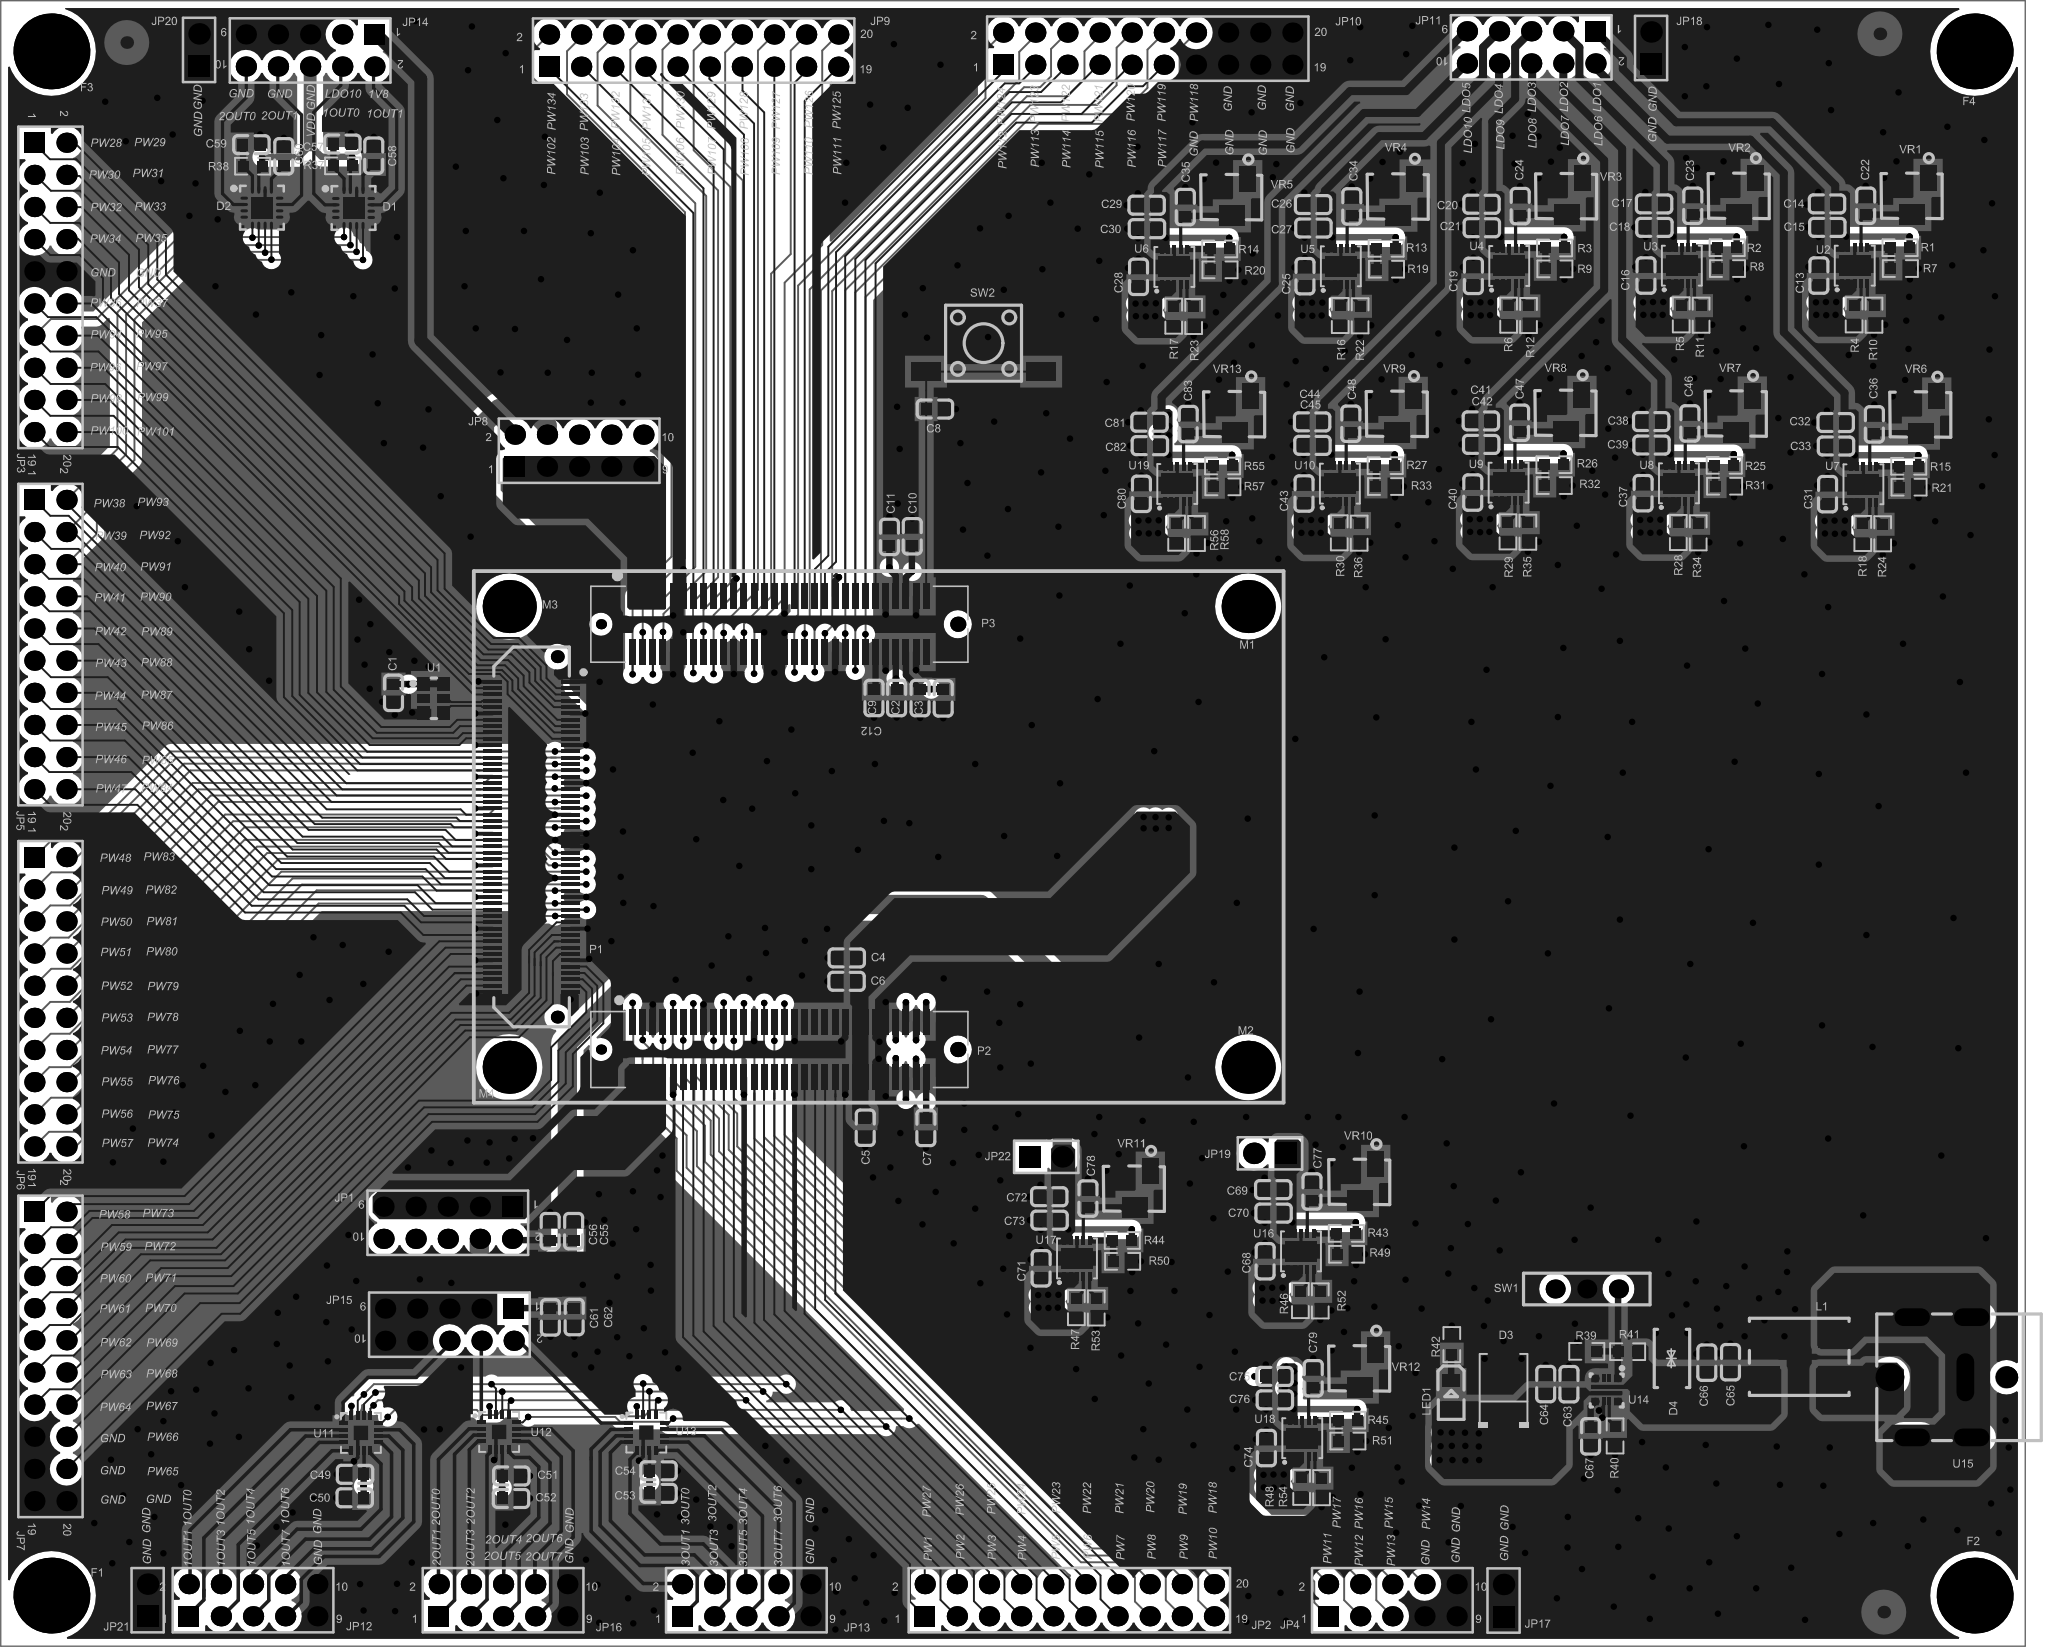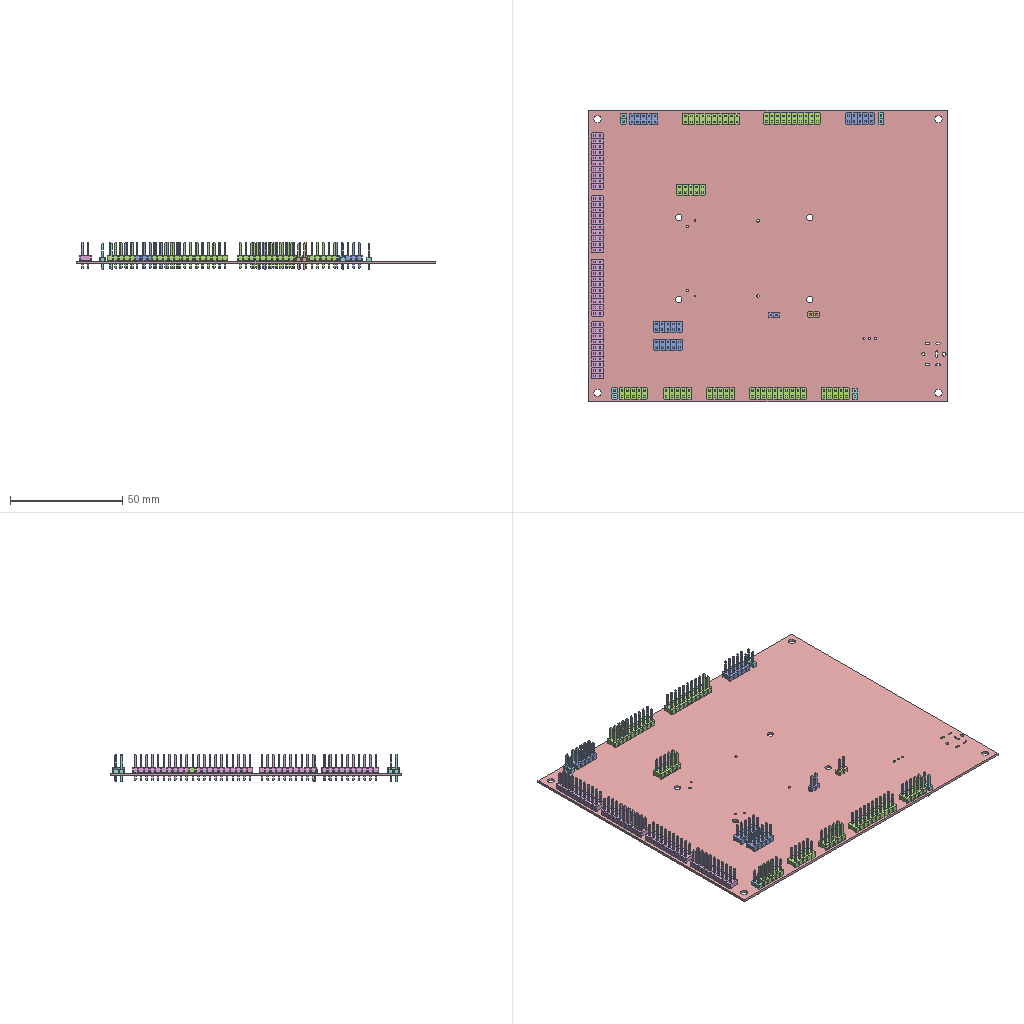Circuit board layout | Altium Designer | box 160 x 130 x 12.2 mm
Layer stack:
# Altium Designer layer stack of  (unit mm; dielectric type: 0 none, 1 core, 2 prepreg, 3 surface material)
index,name,kind,layer,copper_thickness_mm,dielectric_type,dielectric_thickness_mm,dielectric_material,dielectric_constant
0,Top Paste,other,,,,,,
1,Top Overlay,other,,,,,,
2,Top Solder,dielectric,,,3,0.0102,Solder Resist,3.5
3,Top Layer,copper,Top Layer,0.0356,,,,
4,Dielectric1,dielectric,,,1,0.32,FR-4,4.8
5,GND,copper,GND,0.0356,,,,
6,Dielectric2,dielectric,,,2,0.32,FR-4,4.8
7,POWER,copper,POWER,0.0356,,,,
8,Dielectric3,dielectric,,,1,0.32,FR-4,4.8
9,Bottom Layer,copper,Bottom Layer,0.0356,,,,
10,Bottom Solder,dielectric,,,3,0.0102,Solder Resist,3.5
11,Bottom Overlay,other,,,,,,
12,Bottom Paste,other,,,,,,
# drill layer pairs: low layer,high layer
drill_pair,Top Layer,Bottom Layer
Part placement:
Designator,Comment,Layer,Footprint,Center-X(mm),Center-Y(mm),Rotation
C1,X7R  100nF/16V,TopLayer,C0603,31.039,75.311,270
C2,100nF/50V,TopLayer,C0603,72.66,74.915,90
C3,22uF/10V,TopLayer,C0603,74.489,74.889,90
C4,100nF/50V,TopLayer,C0603,66.868,54.372,360
C5,22uF/10V,TopLayer,C0603,68.326,40.97,90
C6,100nF/50V,TopLayer,C0603,66.853,52.527,360
C7,100nF/50V,TopLayer,C0603,73.117,40.955,90
C8,100nF,TopLayer,C0603,73.838,97.739,360
C9,100nF/50V,TopLayer,C0603,70.806,74.915,90
C10,100nF/50V,TopLayer,C0603,72.034,87.681,270
C11,22uF/10V,TopLayer,C0603,70.231,87.63,270
C12,100nF/50V,TopLayer,C0603,69.012,74.905,270
C13,10uF,TopLayer,C0603,143.688,108.28,270
C14,10uF,TopLayer,C0603,144.34,113.944,360
C15,10uF,TopLayer,C0603,144.366,112.09,360
C16,10uF,TopLayer,C0603,130.023,108.28,270
C17,10uF,TopLayer,C0603,130.675,113.944,360
C18,10uF,TopLayer,C0603,130.701,112.09,360
C19,10uF,TopLayer,C0603,116.383,108.255,270
C20,10uF,TopLayer,C0603,117.035,113.919,360
C21,10uF,TopLayer,C0603,117.061,112.065,360
C22,4.7uF,TopLayer,C0603,147.388,113.792,270
C23,4.7uF,TopLayer,C0603,133.723,113.792,270
C24,4.7uF,TopLayer,C0603,120.083,113.767,270
C25,10uF,TopLayer,C0603,103.073,108.229,270
C26,10uF,TopLayer,C0603,103.726,113.894,360
C27,10uF,TopLayer,C0603,103.751,112.039,360
C28,10uF,TopLayer,C0603,89.916,108.179,270
C29,10uF,TopLayer,C0603,90.569,113.843,360
C30,10uF,TopLayer,C0603,90.594,111.989,360
C31,10uF,TopLayer,C0603,144.374,91.008,270
C32,10uF,TopLayer,C0603,145.026,96.672,360
C33,10uF,TopLayer,C0603,145.052,94.818,360
C34,4.7uF,TopLayer,C0603,106.774,113.741,270
C35,4.7uF,TopLayer,C0603,93.617,113.69,270
C36,4.7uF,TopLayer,C0603,148.074,96.52,270
C37,10uF,TopLayer,C0603,129.794,91.084,270
C38,10uF,TopLayer,C0603,130.447,96.749,360
C39,10uF,TopLayer,C0603,130.472,94.894,360
C40,10uF,TopLayer,C0603,116.332,91.135,270
C41,10uF,TopLayer,C0603,116.985,96.799,360
C42,10uF,TopLayer,C0603,117.01,94.945,360
C43,10uF,TopLayer,C0603,102.997,91.059,270
C44,10uF,TopLayer,C0603,103.65,96.723,360
C45,10uF,TopLayer,C0603,103.675,94.869,360
C46,4.7uF,TopLayer,C0603,133.495,96.596,270
C47,4.7uF,TopLayer,C0603,120.033,96.647,270
C48,4.7uF,TopLayer,C0603,106.698,96.571,270
C49,10uF,TopLayer,C0603,28.007,13.574,360
C50,100nF,TopLayer,C0603,27.982,11.72,360
C51,10uF,TopLayer,C0603,40.344,13.452,180
C52,100nF,TopLayer,C0603,40.319,11.674,180
C53,10uF,TopLayer,C0603,51.978,12.08,180
C54,100nF,TopLayer,C0603,51.978,13.858,180
C55,0.1uF/16V,TopLayer,C0603,45.272,32.781,270
C56,0.1uF/16V,TopLayer,C0603,43.418,32.781,270
C57,100nF,TopLayer,C0603,26.991,118.679,180
C58,1.5uF,TopLayer,C0603,29.48,117.765,90
C59,100nF,TopLayer,C0603,19.803,118.628,180
C60,1.5uF,TopLayer,C0603,22.368,117.714,90
C61,10uF,TopLayer,C0603,43.443,25.985,90
C62,10nF,TopLayer,C0603,45.323,26.011,90
C63,22uF/10V,TopLayer,C0603,123.936,20.691,270
C64,22uF/10V,TopLayer,C0603,122.098,20.701,270
C65,X7R 100nF/25V,TopLayer,C0603,136.703,22.428,270
C66,X7R 100nF/25V,TopLayer,C0603,134.832,22.393,270
C67,X7R,TopLayer,C0603,125.654,16.586,90
C68,10uF,TopLayer,C0603,99.924,30.404,270
C69,10uF,TopLayer,C0603,100.576,36.068,360
C70,10uF,TopLayer,C0603,100.602,34.214,360
C71,10uF,TopLayer,C0603,82.22,29.845,270
C72,10uF,TopLayer,C0603,82.872,35.509,360
C73,10uF,TopLayer,C0603,82.898,33.655,360
C74,10uF,TopLayer,C0603,100.025,15.646,270
C75,10uF,TopLayer,C0603,100.678,21.311,360
C76,10uF,TopLayer,C0603,100.703,19.456,360
C77,4.7uF,TopLayer,C0603,103.624,35.916,270
C78,4.7uF,TopLayer,C0603,85.92,35.357,270
C79,4.7uF,TopLayer,C0603,103.726,21.158,270
C80,10uF,TopLayer,C0603,90.145,91.034,270
C81,10uF,TopLayer,C0603,90.797,96.698,360
C82,10uF,TopLayer,C0603,90.823,94.844,360
C83,4.7uF,TopLayer,C0603,93.845,96.545,270
D1,DAC53202,TopLayer,WQFN-16(3x3),27.88,113.624,360
D2,DAC53202,TopLayer,WQFN-16(3x3),20.641,113.65,360
D3,#NAME?,TopLayer,SMB_L4.6-W3.6-LS5.3-RD,118.77,20.345,90
D4,#NAME?,TopLayer,SMA_L4.2-W2.7-LS5.0-BI,132.08,22.733,270
F1,M3,TopLayer,M3,4.004,3.998,0
F2,M3,TopLayer,M3,156.004,3.998,0
F3,M3,TopLayer,M3,4.004,125.998,0
F4,M3,TopLayer,M3,156.004,125.998,0
JP1,Header 5X2,TopLayer,HDR2.54-LI-2x5P,35.331,33.452,180
JP2,Header 2X10,TopLayer,HDR2.54-LI-2x10P,84.455,3.632,360
JP3,Header 2X10,TopLayer,HDR2.54-LI-2x10P,3.928,107.351,270
JP4,Header 5X2,TopLayer,HDR2.54-LI-2x5P,109.982,3.632,360
JP5,Header 2X10,TopLayer,HDR2.54-LI-2x10P,3.928,79.131,270
JP6,Header 2X10,TopLayer,HDR2.54-LI-2x10P,3.928,50.912,270
JP7,Header 2X10,TopLayer,HDR2.54-LI-2x10P,3.928,22.896,270
JP8,Header 5X2,TopLayer,HDR2.54-LI-2x5P,45.711,94.447,360
JP9,Header 2X10,TopLayer,HDR2.54-LI-2x10P,54.762,126.06,360
JP10,Header 2X10,TopLayer,HDR2.54-LI-2x10P,90.653,126.213,360
JP11,Header 5X2,TopLayer,HDR2.54-LI-2x5P,120.955,126.314,180
JP12,Header 5X2,TopLayer,HDR2.54-LI-2x5P,19.939,3.632,360
JP13,Header 5X2,TopLayer,HDR2.54-LI-2x5P,58.928,3.632,360
JP14,Header 5X2,TopLayer,HDR2.54-LI-2x5P,24.451,126.07,180
JP15,Header 5X2,TopLayer,HDR2.54-LI-2x5P,35.458,25.4,180
JP16,Header 5X2,TopLayer,HDR2.54-LI-2x5P,39.7,3.632,360
JP17,HDR-1X2,TopLayer,HDR2.54-LI-2P,118.77,3.607,90
JP18,HDR-1X2,TopLayer,HDR2.54-LI-2P,130.429,126.263,90
JP19,HDR-1X2,TopLayer,HDR2.54-LI-2P,100.305,38.938,180
JP20,HDR-1X2,TopLayer,HDR2.54-LI-2P,15.672,126.111,90
JP21,HDR-1X2,TopLayer,HDR2.54-LI-2P,11.608,3.632,90
JP22,HDR-1X2,TopLayer,HDR2.54-LI-2P,82.626,38.659,360
L1,#NAME?,TopLayer,FILTER-SMD_4P-L7.0-W6.0-TL_SMCM7060,142.138,22.86,180
LED1,#NAME?,TopLayer,LED0805-R-RD,114.63,19.914,270
M1,M2-4-L5-1.6,TopLayer,M2.9,98.587,82.138,0
M2,M2-4-L5-1.6,TopLayer,M2.9,98.587,45.738,0
M3,M2-4-L5-1.6,TopLayer,M2.9,40.187,82.138,0
M4,M2-4-L5-1.6,TopLayer,M2.9,40.187,45.738,0
P1,XMS6302-B,TopLayer,XMS6302-B,41.952,63.938,270
P2,XMS6302-A,TopLayer,XMS6302-A,61.537,47.139,360
P3,XMS6302-C,TopLayer,XMS6302-C,61.537,80.739,360
R1,453k,TopLayer,R0603,150.106,110.49,360
R2,453k,TopLayer,R0603,136.441,110.49,360
R3,453k,TopLayer,R0603,122.801,110.465,360
R4,200k,TopLayer,R0603,146.474,105.181,270
R5,200k,TopLayer,R0603,132.809,105.181,270
R6,200k,TopLayer,R0603,119.169,105.156,270
R7,50k,TopLayer,R0603,150.132,108.839,180
R8,50k,TopLayer,R0603,136.466,108.839,180
R9,50k,TopLayer,R0603,122.827,108.814,180
R10,249R,TopLayer,R0603,148.049,105.156,90
R11,249R,TopLayer,R0603,134.384,105.156,90
R12,249R,TopLayer,R0603,120.744,105.131,90
R13,453k,TopLayer,R0603,109.492,110.439,360
R14,453k,TopLayer,R0603,96.334,110.388,360
R15,453k,TopLayer,R0603,150.792,93.218,360
R16,200k,TopLayer,R0603,105.859,105.131,270
R17,200k,TopLayer,R0603,92.702,105.08,270
R18,200k,TopLayer,R0603,147.16,87.909,270
R19,50k,TopLayer,R0603,109.517,108.788,180
R20,50k,TopLayer,R0603,96.36,108.737,180
R21,50k,TopLayer,R0603,150.817,91.567,180
R22,249R,TopLayer,R0603,107.434,105.105,90
R23,249R,TopLayer,R0603,94.277,105.054,90
R24,249R,TopLayer,R0603,148.735,87.884,90
R25,453k,TopLayer,R0603,136.212,93.294,360
R26,453k,TopLayer,R0603,122.75,93.345,360
R27,453k,TopLayer,R0603,109.415,93.269,360
R28,200k,TopLayer,R0603,132.58,87.986,270
R29,200k,TopLayer,R0603,119.118,88.036,270
R30,200k,TopLayer,R0603,105.783,87.96,270
R31,50k,TopLayer,R0603,136.238,91.643,180
R32,50k,TopLayer,R0603,122.776,91.694,180
R33,50k,TopLayer,R0603,109.441,91.618,180
R34,249R,TopLayer,R0603,134.155,87.96,90
R35,249R,TopLayer,R0603,120.693,88.011,90
R36,249R,TopLayer,R0603,107.358,87.935,90
R37,10K,TopLayer,R0603,27.016,116.952,360
R38,10K,TopLayer,R0603,19.904,116.926,360
R39,357K,TopLayer,R0603,125.349,23.292,180
R40,681O,TopLayer,R0603,127.584,16.612,270
R41,1M,TopLayer,R0603,128.575,23.266,180
R42,10K,TopLayer,R0603,114.681,23.825,270
R43,453k,TopLayer,R0603,106.342,32.614,360
R44,453k,TopLayer,R0603,88.638,32.055,360
R45,453k,TopLayer,R0603,106.444,17.856,360
R46,200k,TopLayer,R0603,102.71,27.305,270
R47,200k,TopLayer,R0603,85.006,26.746,270
R48,200k,TopLayer,R0603,102.811,12.548,270
R49,50k,TopLayer,R0603,106.367,30.963,180
R50,50k,TopLayer,R0603,88.664,30.404,180
R51,50k,TopLayer,R0603,106.469,16.205,180
R52,249R,TopLayer,R0603,104.285,27.28,90
R53,249R,TopLayer,R0603,86.581,26.721,90
R54,249R,TopLayer,R0603,104.386,12.522,90
R55,453k,TopLayer,R0603,96.563,93.243,360
R56,200k,TopLayer,R0603,92.931,87.935,270
R57,50k,TopLayer,R0603,96.588,91.592,180
R58,249R,TopLayer,R0603,94.506,87.909,90
SW1,#NAME?,TopLayer,SW-TH_K3-1204D,125.349,28.219,360
SW2,Key_SMD_6x6x6.5,TopLayer,SW-SMD_4P-L6.0-W6.0-P4.50-LS9.0-2,77.673,102.946,360
U1,SiT9121AI-2B1-XXE100,TopLayer,3225-6p,34.23,74.889,270
U2,#NAME?,TopLayer,DFN-10_L3.0-W3.0-P0.50-BL-EP-3,146.525,109.068,360
U3,#NAME?,TopLayer,DFN-10_L3.0-W3.0-P0.50-BL-EP-3,132.86,109.068,360
U4,#NAME?,TopLayer,DFN-10_L3.0-W3.0-P0.50-BL-EP-3,119.22,109.042,360
U5,#NAME?,TopLayer,DFN-10_L3.0-W3.0-P0.50-BL-EP-3,105.91,109.017,360
U6,#NAME?,TopLayer,DFN-10_L3.0-W3.0-P0.50-BL-EP-3,92.753,108.966,360
U7,#NAME?,TopLayer,DFN-10_L3.0-W3.0-P0.50-BL-EP-3,147.211,91.796,360
U8,#NAME?,TopLayer,DFN-10_L3.0-W3.0-P0.50-BL-EP-3,132.631,91.872,360
U9,#NAME?,TopLayer,DFN-10_L3.0-W3.0-P0.50-BL-EP-3,119.169,91.923,360
U10,#NAME?,TopLayer,DFN-10_L3.0-W3.0-P0.50-BL-EP-3,105.834,91.846,360
U11,DAC60508ZRTER,TopLayer,WQFN-16_L3.0-W3.0-P0.50-BL-EP0.8,28.464,16.85,270
U12,DAC60508ZRTER,TopLayer,WQFN-16_L3.0-W3.0-P0.50-BL-EP0.8,39.386,16.927,270
U13,DAC60508ZRTER,TopLayer,WQFN-16_L3.0-W3.0-P0.50-BL-EP0.8,51.019,16.876,270
U14,#NAME?,TopLayer,VQFN-10_L2.0-W2.0-P0.45-TL,126.898,20.244,270
U15,#NAME?,TopLayer,DC-IN-TH_HX-DC007B-2.5,153.893,21.245,180
U16,#NAME?,TopLayer,DFN-10_L3.0-W3.0-P0.50-BL-EP-3,102.761,31.191,360
U17,#NAME?,TopLayer,DFN-10_L3.0-W3.0-P0.50-BL-EP-3,85.057,30.632,360
U18,#NAME?,TopLayer,DFN-10_L3.0-W3.0-P0.50-BL-EP-3,102.862,16.434,360
U19,#NAME?,TopLayer,DFN-10_L3.0-W3.0-P0.50-BL-EP-3,92.982,91.821,360
VR1,50kO,TopLayer,RES-ADJ-SMD_3224W,151.071,114.554,180
VR2,50kO,TopLayer,RES-ADJ-SMD_3224W,137.406,114.554,180
VR3,50kO,TopLayer,RES-ADJ-SMD_3224W,123.766,114.529,180
VR4,50kO,TopLayer,RES-ADJ-SMD_3224W,110.457,114.503,180
VR5,50kO,TopLayer,RES-ADJ-SMD_3224W,97.3,114.452,180
VR6,50kO,TopLayer,RES-ADJ-SMD_3224W,151.757,97.282,180
VR7,50kO,TopLayer,RES-ADJ-SMD_3224W,137.178,97.358,180
VR8,50kO,TopLayer,RES-ADJ-SMD_3224W,123.716,97.409,180
VR9,50kO,TopLayer,RES-ADJ-SMD_3224W,110.381,97.333,180
VR10,50kO,TopLayer,RES-ADJ-SMD_3224W,107.417,36.652,180
VR11,50kO,TopLayer,RES-ADJ-SMD_3224W,89.603,36.119,180
VR12,50kO,TopLayer,RES-ADJ-SMD_3224W,107.409,21.92,180
VR13,50kO,TopLayer,RES-ADJ-SMD_3224W,97.528,97.307,180
Pad and via stacks:
# Altium Designer via and pad stacks of  (unit mm). Each distinct definition once, with the count of objects using it.
# via: kind,start_layer,end_layer,hole_mm,diameter_mm,mode(0 simple;1 top-mid-bottom;2 full stack),diameter_per_layer,count,example_net
# pad: kind,layer,hole_mm,hole_type(0 round;1 square;2 slot),plating,top_size,top_shape(1 round;2 rect;3 octagon;9 rounded rect),mid_size,bottom_size,mode,footprint,size_per_layer,count,example
pad,Top Layer,0,0,plated,1x1,1,1x1,1x1,0,,,3,MARK
pad,Top Layer,0,0,plated,0.6x0.24,1,0.6x0.24,0.6x0.24,0,WQFN-16(3x3),,16,D2.1
pad,Top Layer,0,0,plated,0.24x0.6,1,0.24x0.6,0.24x0.6,0,WQFN-16(3x3),,16,D2.5
pad,Top Layer,0,0,plated,1.68x1.68,2,1.68x1.68,1.68x1.68,0,WQFN-16(3x3),,2,D2.17
pad,Top Layer,0,0,plated,0.8x0.9,2,0.8x0.9,0.8x0.9,0,C0603,,166,C61.2
pad,Top Layer,0,0,plated,0.8065x0.864,2,0.8065x0.864,0.8065x0.864,0,R0603,,116,R38.2
pad,Top Layer,0,0,plated,0.8x0.8,2,0.8x0.8,0.8x0.8,0,WQFN-16_L3.0-W3.0-P0.50-BL-EP0.8,,3,U13.17
pad,Top Layer,0,0,plated,0.665x0.28,2,0.665x0.28,0.665x0.28,0,WQFN-16_L3.0-W3.0-P0.50-BL-EP0.8,,24,U13.16
pad,Top Layer,0,0,plated,0.28x0.665,2,0.28x0.665,0.28x0.665,0,WQFN-16_L3.0-W3.0-P0.50-BL-EP0.8,,24,U13.12
pad,Top Layer,0,0,plated,1.6x2,2,1.6x2,1.6x2,0,RES-ADJ-SMD_3224W,,13,VR1.2
pad,Top Layer,0,0,plated,2x1.3,2,2x1.3,2x1.3,0,RES-ADJ-SMD_3224W,,26,VR1.3
pad,Top Layer,0,0,plated,2.5x1.6,2,2.5x1.6,2.5x1.6,0,DFN-10_L3.0-W3.0-P0.50-BL-EP-3,,13,U2.11
pad,Top Layer,0,0,plated,0.25x0.65,2,0.25x0.65,0.25x0.65,0,DFN-10_L3.0-W3.0-P0.50-BL-EP-3,,130,U2.10
pad,Top Layer,0,0,plated,2.3x1.5,2,2.3x1.5,2.3x1.5,0,SW-SMD_4P-L6.0-W6.0-P4.50-LS9.0-2,,4,SW2.1
pad,Top Layer,0,0,unplated,0.5x2,2,0.5x2,0.5x2,0,XMS6302-C,,60,P3.C1
pad,Top Layer,0,0,unplated,0.5x2,2,0.5x2,0.5x2,0,XMS6302-A,,60,P2.A3
pad,Top Layer,0,0,plated,0.65x1,2,0.65x1,0.65x1,0,3225-6p,,2,U1.2
pad,Top Layer,0,0,plated,1.05x1,2,1.05x1,1.05x1,0,3225-6p,,4,U1.1
pad,Top Layer,0,0,plated,0.3051x1.448,2,0.3051x1.448,0.3051x1.448,0,XMS6302-B,,100,P1.B36
pad,Top Layer,0,0,plated,2x1.8,2,2x1.8,2x1.8,0,SMA_L4.2-W2.7-LS5.0-BI,,2,D4.2
pad,Top Layer,0,0,plated,2.5x1.75,2,2.5x1.75,2.5x1.75,0,FILTER-SMD_4P-L7.0-W6.0-TL_SMCM7060,,4,L1.1
pad,Top Layer,0,0,plated,2.047x2.192,2,2.047x2.192,2.047x2.192,0,SMB_L4.6-W3.6-LS5.3-RD,,2,D3.1
pad,Top Layer,0,0,plated,1x1.399,2,1x1.399,1x1.399,0,LED0805-R-RD,,2,LED1.1
pad,Top Layer,0,0,plated,0.6x0.6,1,0.6x0.6,0.6x0.6,0,VQFN-10_L2.0-W2.0-P0.45-TL,,4,U14.1
pad,Top Layer,0,0,plated,0.3x2.4,2,0.3x2.4,0.3x2.4,0,VQFN-10_L2.0-W2.0-P0.45-TL,,2,U14.5
pad,Top Layer,0,0,plated,0.25x0.6,2,0.25x0.6,0.25x0.6,0,VQFN-10_L2.0-W2.0-P0.45-TL,,4,U14.2
pad,Multi-Layer,0.9,0,plated,1.6x1.6,1,1.6x1.6,1.6x1.6,0,HDR2.54-LI-2x5P,,81,JP15.10
pad,Multi-Layer,0.9,0,plated,1.6x1.6,2,1.6x1.6,1.6x1.6,0,HDR2.54-LI-2x5P,,9,JP15.1
pad,Multi-Layer,3.2,0,plated,6x6,1,6x6,6x6,0,M3,,4,F1.1
pad,Multi-Layer,0.9,0,plated,1.6x1.6,1,1.6x1.6,1.6x1.6,0,HDR2.54-LI-2x10P,,133,JP10.20
pad,Multi-Layer,0.9,0,plated,1.6x1.6,2,1.6x1.6,1.6x1.6,0,HDR2.54-LI-2x10P,,7,JP10.1
pad,Multi-Layer,1.2,0,unplated,1.2x1.2,1,1.2x1.2,1.2x1.2,0,XMS6302-C,,1,P3.
pad,Multi-Layer,0.8,0,unplated,0.8x0.8,1,0.8x0.8,0.8x0.8,0,XMS6302-C,,1,P3.
pad,Multi-Layer,0.8,0,unplated,0.8x0.8,1,0.8x0.8,0.8x0.8,0,XMS6302-A,,1,P2.
pad,Multi-Layer,1.2,0,unplated,1.2x1.2,1,1.2x1.2,1.2x1.2,0,XMS6302-A,,1,P2.
pad,Multi-Layer,1.016,0,unplated,1.016x1.016,1,1.016x1.016,1.016x1.016,0,XMS6302-B,,2,P1.
pad,Multi-Layer,0.9,0,plated,1.7x1.7,2,1.7x1.7,1.7x1.7,0,HDR2.54-LI-2P,,6,JP20.1
pad,Multi-Layer,0.9,0,plated,1.7x1.7,1,1.7x1.7,1.7x1.7,0,HDR2.54-LI-2P,,6,JP20.2
pad,Multi-Layer,2.9,0,plated,4.2x4.2,1,4.2x4.2,4.2x4.2,0,M2.9,,4,M3.1
pad,Multi-Layer,1.7,0,unplated,1.7x1.7,1,1.7x1.7,1.7x1.7,0,DC-IN-TH_HX-DC007B-2.5,,1,U15.0
pad,Multi-Layer,1.4,0,plated,2.2x2.2,1,2.2x2.2,2.2x2.2,0,DC-IN-TH_HX-DC007B-2.5,,1,U15.1
pad,Multi-Layer,0.8,2,plated,1.4x3.8,1,1.4x3.8,1.4x3.8,0,DC-IN-TH_HX-DC007B-2.5,,1,U15.2
pad,Multi-Layer,0.8,2,plated,1.4x2.8,1,1.4x2.8,1.4x2.8,0,DC-IN-TH_HX-DC007B-2.5,,4,U15.3
pad,Multi-Layer,1,0,plated,1.5x1.5,1,1.5x1.5,1.5x1.5,0,SW-TH_K3-1204D,,3,SW1.3
via,Top Layer,Bottom Layer,0.3048,0.508,0,,1218,GND
Copper pours:
name,layer,net,type(0 solid;1 hatched;2 none)
Bottom Layer-No Net,Top Layer,GND,0
Bottom Layer-No Net,Top Layer,VCC3V3D,0
Bottom Layer-No Net,Top Layer,VCC5VD,0
Bottom Layer-No Net,Top Layer,NetC65_2,0
Bottom Layer-No Net,Top Layer,NetL1_2,0
Bottom Layer-No Net,Top Layer,NetL1_1,0
Bottom Layer-No Net,Top Layer,VCC1V8D,0
Bottom Layer-No Net,Top Layer,VCC5VD,0
Bottom Layer-No Net,Top Layer,VCC5VD,0
Bottom Layer-No Net,Top Layer,VCC5VD,0
Bottom Layer-No Net,Top Layer,VCC5VD,0
Bottom Layer-No Net,Top Layer,LDO_6,0
Bottom Layer-No Net,Top Layer,VCC5VD,0
Bottom Layer-No Net,Top Layer,LDO_7,0
Bottom Layer-No Net,Top Layer,VCC5VD,0
Bottom Layer-No Net,Top Layer,LDO_8,0
Bottom Layer-No Net,Top Layer,VCC5VD,0
Bottom Layer-No Net,Top Layer,LDO_9,0
Bottom Layer-No Net,Top Layer,VCC5VD,0
Bottom Layer-No Net,Top Layer,LDO_10,0
Bottom Layer-No Net,Top Layer,LDO_1,0
Bottom Layer-No Net,Top Layer,VCC5VD,0
Bottom Layer-No Net,Top Layer,LDO_2,0
Bottom Layer-No Net,Top Layer,VCC5VD,0
Bottom Layer-No Net,Top Layer,LDO_3,0
Bottom Layer-No Net,Top Layer,VCC5VD,0
Bottom Layer-No Net,Top Layer,VCC5VD,0
Bottom Layer-No Net,Top Layer,LDO_4,0
Bottom Layer-No Net,Top Layer,LDO_5,0
Bottom Layer-No Net,Top Layer,VCC5VD,0
Bottom Layer-No Net,Top Layer,NetJP8_1,0
Bottom Layer-No Net,Top Layer,NetJP1_1,0
Bottom Layer-No Net,Top Layer,VCC3V3D,0
Bottom Layer-No Net,Top Layer,VCC2V5D,0
Bottom Layer-No Net,Bottom Layer,GND,0
Design rules, without the lines most boards share:
# Altium Designer design rules of  (exported by Altium Designer, unit mm)
# columns: name | kind | enabled | priority | scope1 | scope2 | descriptor | typed fields (field=value)
Clearance_2 | 0 | enabled | 1 | HASPAD('FREE-MARK') | All | Clearance Constraint (Gap=1.27mm) (HASPAD('FREE-MARK')),(All) | gap=1.27
Clearance_1 | 0 | enabled | 2 | INPOLYGON | All | Clearance Constraint (Gap=0.152mm) (INPOLYGON),(All) | gap=0.1524
Clearance | 0 | enabled | 3 | All | All | Clearance Constraint (Gap=0.152mm) (All),(All) | gap=0.1524
PlaneConnect | 6 | enabled | 1 | All | All | Power Plane Connect Rule(Direct Connect )(Expansion=0.508mm) (Conductor Width=0.254mm) (Air Gap=0.254mm) (Entries=4) (All) | relief_conductor_width=0.254 relief_entries=4 relief_expansion=0.508
PlaneClearance | 12 | enabled | 1 | All | All | Power Plane Clearance (Clearance =0.152mm) (All) | clearance=0.1524
PolygonConnect | 20 | enabled | 1 | All | All | Polygon Connect Rule(Direct Connect )(Conductor Width=0.254mm) (Relief Angle=90 Angle) (Entries=4) (Air Gap Width=0.254mm) (All),(All) | connect_style(0=relief,1=direct,2=none)=1 relief_conductor_width=0.254 relief_entries=4
Width | 2 | enabled | 1 | All | All | Width Constraint (Min=0.152mm) (Max=2.032mm) (Preferred=0.152mm) (All) |
RoutingCorners | 10 | enabled | 1 | All | All | Routing Corners (Style=45-Degree) (Min Setback=2.54mm) (Max Setback=2.54mm) (All) |
RoutingVias | 11 | enabled | 1 | All | All | Routing Via (MinHoleWidth=0.305mm) (MaxHoleWidth=0.305mm) (PreferredHoleWidth=0.305mm) (MinWidth=0.508mm) (MaxWidth=0.508mm) (PreferedWidth=0.508mm) (All) | via_min_hole=0.3048 via_max_hole=0.3048 via_preferred_diameter=0.508 via_preferred_hole=0.3048
PasteMaskExpansion | 14 | enabled | 1 | All | All | Paste Mask Expansion (Expansion =0mm) (All) | expansion=0
SolderMaskExpansion | 13 | enabled | 1 | All | All | Solder Mask Expansion (Expansion =0.102mm) (All) | expansion=0.1016
ComponentClearance | 24 | enabled | 1 | All | All | Component Clearance Constraint ( Horizontal Gap = 0.254mm, Vertical Gap = 0.254mm ) (All),(All)  | gap=0.254
Height | 50 | enabled | 1 | All | All | Height Constraint (Min=0mm) (Max=25.4mm) (Prefered=12.7mm) (All) | min_height=0 max_height=25.4
HoleSize | 42 | enabled | 1 | All | All | Hole Size Constraint (Min=0.025mm) (Max=12.7mm) (All) |
DiffPairsRouting | 51 | enabled | 1 | All | All | Differential Pairs Uncoupled Length using the Gap Constraints (Min=0.152mm) (Max=0.152mm) (Prefered=0.152mm)  and Width Constraints (Min=0.381mm) (Max=0.381mm) (Prefered=0.381mm) (All) |
HoleToHoleClearance | 52 | enabled | 1 | All | All | Hole To Hole Clearance (Gap=0mm) (All),(All) | gap=0
MinimumSolderMaskSliver | 53 | enabled | 1 | All | All | Minimum Solder Mask Sliver (Gap=0mm) (All),(All) |
SilkscreenOverComponentPads | 54 | enabled | 1 | IsPad | All | Silk To Solder Mask (Clearance=0mm) (IsPad),(All) |
SilkToSilkClearance | 55 | enabled | 1 | All | All | Silk to Silk (Clearance=0mm) (All),(All) |
NetAntennae | 56 | enabled | 1 | All | All | Net Antennae (Tolerance=0mm) (All) |
Classes set for this board:
# Altium Designer classes of  (member kind: 0 net, 1 component, 2 from-to, 3 pad, 4 layer, 5 differential pair, 6 design channel, 7 polygon, 8 structure, 9 xSignal)
# columns: class name | member kind | superclass | members
AnalogSignal | 1 | no | C13; C14; C15; C16; C17; C18; C19; C20; C21; C22; C23; C24; C25; C26; C27; C28; C29; C30; C31; C32; C33; C34; C35; C36; C37; C38; C39; C40; C41; C42; C43; C44; C45; C46; C47; C48; C49; C50; C51; C52; C53; C54; C55; C56; C57; C58; C59; C60; C61; C62; C81; C?; C?; C?; D1; D2; JP11; JP12; JP13; JP14; JP15; JP16; R1; R2; R3; R4; R5; R6; R7; R8; R9; R10; R11; R12; R13; R14; R15; R16; R17; R18; R19; R20; R21; R22; R23; R24; R25; R26; R27; R28; R29; R30; R31; R32; R33; R34; R35; R36; R37; R38; R57; R?; R?; R?; U2; U3; U4; U5; U6; U7; U8; U9; U10; U11; U12; U13; U19; VR1; VR2; VR3; VR4; VR5; VR6; VR7; VR8; VR9; VR13; C81; C82; C83; R55; R56; R58; C80; C13; C14; C15; C16; C17; C18; C19; C20; C21; C22; C23; C24; C25; C26; C27; C28; C29; C30; C31; C32; C33; C34; C35; C36; C37; C38; C39; C40; C41; C42; C43; C44; C45; C46; C47; C48; C49; C50; C51; C52; C53; C54; C55; C56; C57; C58; C59; C60; C61; C62; C80; C81; C82; C83; D1; D2; JP11; JP12; JP13; JP14; JP15; JP16; R1; R2; R3; R4; R5; R6; R7; R8; R9; R10; R11; R12; R13; R14; R15; R16; R17; R18; R19; R20; R21; R22; R23; R24; R25; R26; R27; R28; R29; R30; R31; R32; R33; R34; R35; R36; R37; R38; R55; R56; R57; R58; U2; U3; U4; U5; U6; U7; U8; U9; U10; U11; U12; U13; U19; VR1; VR2; VR3; VR4; VR5; VR6; VR7; VR8; VR9; VR13;
FPGA | 1 | no | C1; C2; C3; C4; C5; C6; C7; C8; C9; C10; C11; C12; F1; F2; F3; F4; JP1; JP2; JP3; JP4; JP5; JP6; JP7; JP8; JP9; JP10; P1; P2; P3; SW2; U1; C1; C2; C3; C4; C5; C6; C7; C8; C9; C10; C11; C12; F1; F2; F3; F4; JP1; JP2; JP3; JP4; JP5; JP6; JP7; JP8; JP9; JP10; P1; P2; P3; SW2; U1;
Power | 1 | no | C63; C64; C65; C66; C67; C68; C69; C70; C71; C72; C73; C74; C75; C76; C77; C78; C79; D3; D4; JP17; JP18; JP19; JP20; JP21; JP22; L1; LED1; M1; M2; M3; M4; R39; R40; R41; R42; R43; R44; R45; R46; R47; R48; R49; R50; R51; R52; R53; R54; SW1; U14; U15; U16; U17; U18; VR10; VR11; VR12; C63; C64; C65; C66; C67; C68; C69; C70; C71; C72; C73; C74; C75; C76; C77; C78; C79; D3; D4; JP17; JP18; JP19; JP20; JP21; JP22; L1; LED1; M1; M2; M3; M4; R39; R40; R41; R42; R43; R44; R45; R46; R47; R48; R49; R50; R51; R52; R53; R54; SW1; U14; U15; U16; U17; U18; VR10; VR11; VR12;